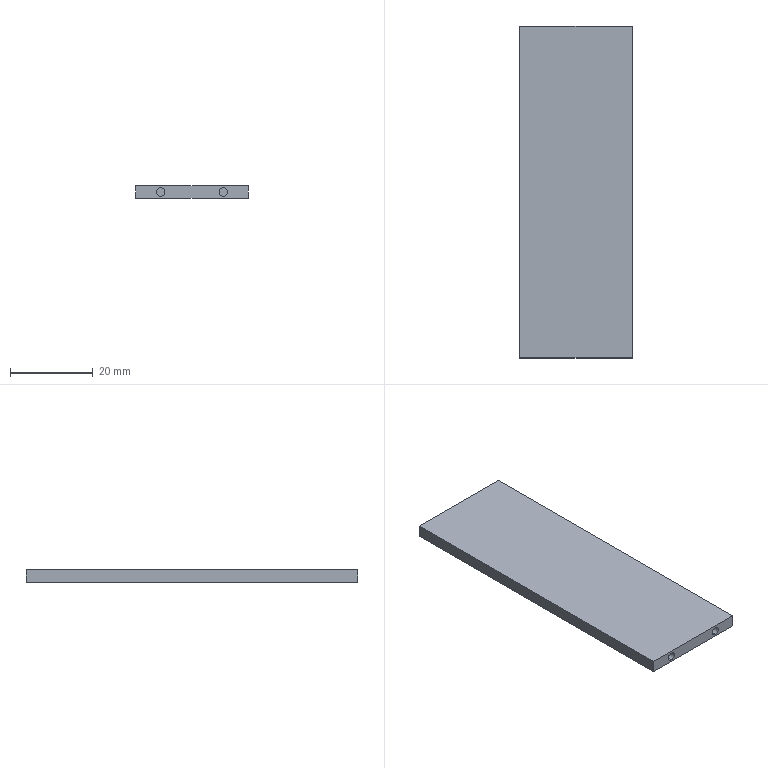Part | SolidWorks | features Cut 1, Extrusion 1 | 1 solid | 12 faces | box 27 x 80 x 3 mm | volume 6449 mm3 | plane 8 | cylinder 4 | commonest cylinder face diameters 2 x4
STEP:
#1=CARTESIAN_POINT('',(-28.957,-53.022,2.5));
#2=VERTEX_POINT('',#1);
#3=CARTESIAN_POINT('',(-28.957,-53.022,0.5));
#4=VERTEX_POINT('',#3);
#5=CARTESIAN_POINT('',(-28.957,-53.022,1.5));
#6=DIRECTION('',(0.,-1.,0.));
#7=DIRECTION('',(0.,0.,-1.));
#8=AXIS2_PLACEMENT_3D('',#5,#6,#7);
#9=CIRCLE('',#8,1.);
#10=EDGE_CURVE('',#2,#4,#9,.T.);
#11=ORIENTED_EDGE('',*,*,#10,.F.);
#12=CARTESIAN_POINT('',(-28.957,-58.022,2.5));
#13=VERTEX_POINT('',#12);
#14=CARTESIAN_POINT('',(-28.957,-53.022,2.5));
#15=DIRECTION('',(0.,-1.,0.));
#16=VECTOR('',#15,1000.);
#17=LINE('',#14,#16);
#18=EDGE_CURVE('',#2,#13,#17,.T.);
#19=ORIENTED_EDGE('',*,*,#18,.T.);
#20=CARTESIAN_POINT('',(-28.957,-58.022,0.5));
#21=VERTEX_POINT('',#20);
#22=CARTESIAN_POINT('',(-28.957,-58.022,1.5));
#23=DIRECTION('',(0.,1.,0.));
#24=DIRECTION('',(0.,0.,1.));
#25=AXIS2_PLACEMENT_3D('',#22,#23,#24);
#26=CIRCLE('',#25,1.);
#27=EDGE_CURVE('',#21,#13,#26,.T.);
#28=ORIENTED_EDGE('',*,*,#27,.F.);
#29=CARTESIAN_POINT('',(-28.957,-53.022,0.5));
#30=DIRECTION('',(0.,-1.,0.));
#31=VECTOR('',#30,1000.);
#32=LINE('',#29,#31);
#33=EDGE_CURVE('',#4,#21,#32,.T.);
#34=ORIENTED_EDGE('',*,*,#33,.F.);
#35=EDGE_LOOP('',(#11,#19,#28,#34));
#36=FACE_OUTER_BOUND('',#35,.T.);
#37=CARTESIAN_POINT('',(-28.957,-53.022,1.5));
#38=DIRECTION('',(0.,-1.,0.));
#39=DIRECTION('',(0.,0.,-1.));
#40=AXIS2_PLACEMENT_3D('',#37,#38,#39);
#41=CYLINDRICAL_SURFACE('',#40,1.);
#42=ADVANCED_FACE('',(#36),#41,.F.);
#43=CARTESIAN_POINT('',(-13.957,-53.022,2.5));
#44=VERTEX_POINT('',#43);
#45=CARTESIAN_POINT('',(-13.957,-53.022,0.5));
#46=VERTEX_POINT('',#45);
#47=CARTESIAN_POINT('',(-13.957,-53.022,1.5));
#48=DIRECTION('',(0.,-1.,0.));
#49=DIRECTION('',(0.,0.,-1.));
#50=AXIS2_PLACEMENT_3D('',#47,#48,#49);
#51=CIRCLE('',#50,1.);
#52=EDGE_CURVE('',#44,#46,#51,.T.);
#53=ORIENTED_EDGE('',*,*,#52,.F.);
#54=CARTESIAN_POINT('',(-13.957,-58.022,2.5));
#55=VERTEX_POINT('',#54);
#56=CARTESIAN_POINT('',(-13.957,-53.022,2.5));
#57=DIRECTION('',(0.,-1.,0.));
#58=VECTOR('',#57,1000.);
#59=LINE('',#56,#58);
#60=EDGE_CURVE('',#44,#55,#59,.T.);
#61=ORIENTED_EDGE('',*,*,#60,.T.);
#62=CARTESIAN_POINT('',(-13.957,-58.022,0.5));
#63=VERTEX_POINT('',#62);
#64=CARTESIAN_POINT('',(-13.957,-58.022,1.5));
#65=DIRECTION('',(0.,1.,0.));
#66=DIRECTION('',(0.,0.,1.));
#67=AXIS2_PLACEMENT_3D('',#64,#65,#66);
#68=CIRCLE('',#67,1.);
#69=EDGE_CURVE('',#63,#55,#68,.T.);
#70=ORIENTED_EDGE('',*,*,#69,.F.);
#71=CARTESIAN_POINT('',(-13.957,-53.022,0.5));
#72=DIRECTION('',(0.,-1.,0.));
#73=VECTOR('',#72,1000.);
#74=LINE('',#71,#73);
#75=EDGE_CURVE('',#46,#63,#74,.T.);
#76=ORIENTED_EDGE('',*,*,#75,.F.);
#77=EDGE_LOOP('',(#53,#61,#70,#76));
#78=FACE_OUTER_BOUND('',#77,.T.);
#79=CARTESIAN_POINT('',(-13.957,-53.022,1.5));
#80=DIRECTION('',(0.,-1.,0.));
#81=DIRECTION('',(0.,0.,-1.));
#82=AXIS2_PLACEMENT_3D('',#79,#80,#81);
#83=CYLINDRICAL_SURFACE('',#82,1.);
#84=ADVANCED_FACE('',(#78),#83,.F.);
#85=ORIENTED_EDGE('',*,*,#27,.T.);
#86=CARTESIAN_POINT('',(-28.957,-58.022,1.5));
#87=DIRECTION('',(0.,1.,0.));
#88=DIRECTION('',(0.,0.,1.));
#89=AXIS2_PLACEMENT_3D('',#86,#87,#88);
#90=CIRCLE('',#89,1.);
#91=EDGE_CURVE('',#13,#21,#90,.T.);
#92=ORIENTED_EDGE('',*,*,#91,.T.);
#93=EDGE_LOOP('',(#85,#92));
#94=FACE_BOUND('',#93,.T.);
#95=ORIENTED_EDGE('',*,*,#69,.T.);
#96=CARTESIAN_POINT('',(-13.957,-58.022,1.5));
#97=DIRECTION('',(0.,1.,0.));
#98=DIRECTION('',(0.,0.,1.));
#99=AXIS2_PLACEMENT_3D('',#96,#97,#98);
#100=CIRCLE('',#99,1.);
#101=EDGE_CURVE('',#55,#63,#100,.T.);
#102=ORIENTED_EDGE('',*,*,#101,.T.);
#103=EDGE_LOOP('',(#95,#102));
#104=FACE_BOUND('',#103,.T.);
#105=CARTESIAN_POINT('',(-34.957,-58.022,0.));
#106=VERTEX_POINT('',#105);
#107=CARTESIAN_POINT('',(-7.957,-58.022,0.));
#108=VERTEX_POINT('',#107);
#109=CARTESIAN_POINT('',(-34.957,-58.022,0.));
#110=DIRECTION('',(1.,0.,0.));
#111=VECTOR('',#110,1000.);
#112=LINE('',#109,#111);
#113=EDGE_CURVE('',#106,#108,#112,.T.);
#114=ORIENTED_EDGE('',*,*,#113,.T.);
#115=CARTESIAN_POINT('',(-7.957,-58.022,3.));
#116=VERTEX_POINT('',#115);
#117=CARTESIAN_POINT('',(-7.957,-58.022,3.));
#118=DIRECTION('',(0.,0.,-1.));
#119=VECTOR('',#118,1000.);
#120=LINE('',#117,#119);
#121=EDGE_CURVE('',#116,#108,#120,.T.);
#122=ORIENTED_EDGE('',*,*,#121,.F.);
#123=CARTESIAN_POINT('',(-34.957,-58.022,3.));
#124=VERTEX_POINT('',#123);
#125=CARTESIAN_POINT('',(-34.957,-58.022,3.));
#126=DIRECTION('',(1.,0.,0.));
#127=VECTOR('',#126,1000.);
#128=LINE('',#125,#127);
#129=EDGE_CURVE('',#124,#116,#128,.T.);
#130=ORIENTED_EDGE('',*,*,#129,.F.);
#131=CARTESIAN_POINT('',(-34.957,-58.022,3.));
#132=DIRECTION('',(0.,0.,-1.));
#133=VECTOR('',#132,1000.);
#134=LINE('',#131,#133);
#135=EDGE_CURVE('',#124,#106,#134,.T.);
#136=ORIENTED_EDGE('',*,*,#135,.T.);
#137=EDGE_LOOP('',(#114,#122,#130,#136));
#138=FACE_OUTER_BOUND('',#137,.T.);
#139=CARTESIAN_POINT('',(-34.957,-58.022,3.));
#140=DIRECTION('',(0.,1.,0.));
#141=DIRECTION('',(0.,0.,1.));
#142=AXIS2_PLACEMENT_3D('',#139,#140,#141);
#143=PLANE('',#142);
#144=ADVANCED_FACE('',(#94,#104,#138),#143,.F.);
#145=CARTESIAN_POINT('',(-7.957,21.978,0.));
#146=VERTEX_POINT('',#145);
#147=CARTESIAN_POINT('',(-7.957,-58.022,0.));
#148=DIRECTION('',(0.,1.,0.));
#149=VECTOR('',#148,1000.);
#150=LINE('',#147,#149);
#151=EDGE_CURVE('',#108,#146,#150,.T.);
#152=ORIENTED_EDGE('',*,*,#151,.T.);
#153=CARTESIAN_POINT('',(-7.957,21.978,3.));
#154=VERTEX_POINT('',#153);
#155=CARTESIAN_POINT('',(-7.957,21.978,3.));
#156=DIRECTION('',(0.,0.,-1.));
#157=VECTOR('',#156,1000.);
#158=LINE('',#155,#157);
#159=EDGE_CURVE('',#154,#146,#158,.T.);
#160=ORIENTED_EDGE('',*,*,#159,.F.);
#161=CARTESIAN_POINT('',(-7.957,-58.022,3.));
#162=DIRECTION('',(0.,1.,0.));
#163=VECTOR('',#162,1000.);
#164=LINE('',#161,#163);
#165=EDGE_CURVE('',#116,#154,#164,.T.);
#166=ORIENTED_EDGE('',*,*,#165,.F.);
#167=ORIENTED_EDGE('',*,*,#121,.T.);
#168=EDGE_LOOP('',(#152,#160,#166,#167));
#169=FACE_OUTER_BOUND('',#168,.T.);
#170=CARTESIAN_POINT('',(-7.957,-58.022,3.));
#171=DIRECTION('',(-1.,0.,0.));
#172=DIRECTION('',(0.,0.,1.));
#173=AXIS2_PLACEMENT_3D('',#170,#171,#172);
#174=PLANE('',#173);
#175=ADVANCED_FACE('',(#169),#174,.F.);
#176=CARTESIAN_POINT('',(-34.957,21.978,0.));
#177=VERTEX_POINT('',#176);
#178=CARTESIAN_POINT('',(-34.957,21.978,0.));
#179=DIRECTION('',(1.,0.,0.));
#180=VECTOR('',#179,1000.);
#181=LINE('',#178,#180);
#182=EDGE_CURVE('',#177,#146,#181,.T.);
#183=ORIENTED_EDGE('',*,*,#182,.F.);
#184=CARTESIAN_POINT('',(-34.957,21.978,3.));
#185=VERTEX_POINT('',#184);
#186=CARTESIAN_POINT('',(-34.957,21.978,3.));
#187=DIRECTION('',(0.,0.,-1.));
#188=VECTOR('',#187,1000.);
#189=LINE('',#186,#188);
#190=EDGE_CURVE('',#185,#177,#189,.T.);
#191=ORIENTED_EDGE('',*,*,#190,.F.);
#192=CARTESIAN_POINT('',(-34.957,21.978,3.));
#193=DIRECTION('',(1.,0.,0.));
#194=VECTOR('',#193,1000.);
#195=LINE('',#192,#194);
#196=EDGE_CURVE('',#185,#154,#195,.T.);
#197=ORIENTED_EDGE('',*,*,#196,.T.);
#198=ORIENTED_EDGE('',*,*,#159,.T.);
#199=EDGE_LOOP('',(#183,#191,#197,#198));
#200=FACE_OUTER_BOUND('',#199,.T.);
#201=CARTESIAN_POINT('',(-34.957,21.978,3.));
#202=DIRECTION('',(0.,1.,0.));
#203=DIRECTION('',(0.,0.,1.));
#204=AXIS2_PLACEMENT_3D('',#201,#202,#203);
#205=PLANE('',#204);
#206=ADVANCED_FACE('',(#200),#205,.T.);
#207=CARTESIAN_POINT('',(-34.957,-58.022,0.));
#208=DIRECTION('',(0.,1.,0.));
#209=VECTOR('',#208,1000.);
#210=LINE('',#207,#209);
#211=EDGE_CURVE('',#106,#177,#210,.T.);
#212=ORIENTED_EDGE('',*,*,#211,.F.);
#213=ORIENTED_EDGE('',*,*,#135,.F.);
#214=CARTESIAN_POINT('',(-34.957,-58.022,3.));
#215=DIRECTION('',(0.,1.,0.));
#216=VECTOR('',#215,1000.);
#217=LINE('',#214,#216);
#218=EDGE_CURVE('',#124,#185,#217,.T.);
#219=ORIENTED_EDGE('',*,*,#218,.T.);
#220=ORIENTED_EDGE('',*,*,#190,.T.);
#221=EDGE_LOOP('',(#212,#213,#219,#220));
#222=FACE_OUTER_BOUND('',#221,.T.);
#223=CARTESIAN_POINT('',(-34.957,-58.022,3.));
#224=DIRECTION('',(-1.,0.,0.));
#225=DIRECTION('',(0.,0.,1.));
#226=AXIS2_PLACEMENT_3D('',#223,#224,#225);
#227=PLANE('',#226);
#228=ADVANCED_FACE('',(#222),#227,.T.);
#229=ORIENTED_EDGE('',*,*,#129,.T.);
#230=ORIENTED_EDGE('',*,*,#165,.T.);
#231=ORIENTED_EDGE('',*,*,#196,.F.);
#232=ORIENTED_EDGE('',*,*,#218,.F.);
#233=EDGE_LOOP('',(#229,#230,#231,#232));
#234=FACE_OUTER_BOUND('',#233,.T.);
#235=CARTESIAN_POINT('',(0.,0.,3.));
#236=DIRECTION('',(0.,0.,1.));
#237=DIRECTION('',(1.,0.,0.));
#238=AXIS2_PLACEMENT_3D('',#235,#236,#237);
#239=PLANE('',#238);
#240=ADVANCED_FACE('',(#234),#239,.T.);
#241=ORIENTED_EDGE('',*,*,#113,.F.);
#242=ORIENTED_EDGE('',*,*,#211,.T.);
#243=ORIENTED_EDGE('',*,*,#182,.T.);
#244=ORIENTED_EDGE('',*,*,#151,.F.);
#245=EDGE_LOOP('',(#241,#242,#243,#244));
#246=FACE_OUTER_BOUND('',#245,.T.);
#247=CARTESIAN_POINT('',(0.,0.,0.));
#248=DIRECTION('',(0.,0.,1.));
#249=DIRECTION('',(1.,0.,0.));
#250=AXIS2_PLACEMENT_3D('',#247,#248,#249);
#251=PLANE('',#250);
#252=ADVANCED_FACE('',(#246),#251,.F.);
#253=ORIENTED_EDGE('',*,*,#60,.F.);
#254=CARTESIAN_POINT('',(-13.957,-53.022,1.5));
#255=DIRECTION('',(0.,-1.,0.));
#256=DIRECTION('',(0.,0.,-1.));
#257=AXIS2_PLACEMENT_3D('',#254,#255,#256);
#258=CIRCLE('',#257,1.);
#259=EDGE_CURVE('',#46,#44,#258,.T.);
#260=ORIENTED_EDGE('',*,*,#259,.F.);
#261=ORIENTED_EDGE('',*,*,#75,.T.);
#262=ORIENTED_EDGE('',*,*,#101,.F.);
#263=EDGE_LOOP('',(#253,#260,#261,#262));
#264=FACE_OUTER_BOUND('',#263,.T.);
#265=CARTESIAN_POINT('',(-13.957,-53.022,1.5));
#266=DIRECTION('',(0.,-1.,0.));
#267=DIRECTION('',(0.,0.,-1.));
#268=AXIS2_PLACEMENT_3D('',#265,#266,#267);
#269=CYLINDRICAL_SURFACE('',#268,1.);
#270=ADVANCED_FACE('',(#264),#269,.F.);
#271=ORIENTED_EDGE('',*,*,#259,.T.);
#272=ORIENTED_EDGE('',*,*,#52,.T.);
#273=EDGE_LOOP('',(#271,#272));
#274=FACE_OUTER_BOUND('',#273,.T.);
#275=CARTESIAN_POINT('',(-13.957,-53.022,1.5));
#276=DIRECTION('',(0.,-1.,0.));
#277=DIRECTION('',(0.,0.,-1.));
#278=AXIS2_PLACEMENT_3D('',#275,#276,#277);
#279=PLANE('',#278);
#280=ADVANCED_FACE('',(#274),#279,.T.);
#281=ORIENTED_EDGE('',*,*,#18,.F.);
#282=CARTESIAN_POINT('',(-28.957,-53.022,1.5));
#283=DIRECTION('',(0.,-1.,0.));
#284=DIRECTION('',(0.,0.,-1.));
#285=AXIS2_PLACEMENT_3D('',#282,#283,#284);
#286=CIRCLE('',#285,1.);
#287=EDGE_CURVE('',#4,#2,#286,.T.);
#288=ORIENTED_EDGE('',*,*,#287,.F.);
#289=ORIENTED_EDGE('',*,*,#33,.T.);
#290=ORIENTED_EDGE('',*,*,#91,.F.);
#291=EDGE_LOOP('',(#281,#288,#289,#290));
#292=FACE_OUTER_BOUND('',#291,.T.);
#293=CARTESIAN_POINT('',(-28.957,-53.022,1.5));
#294=DIRECTION('',(0.,-1.,0.));
#295=DIRECTION('',(0.,0.,-1.));
#296=AXIS2_PLACEMENT_3D('',#293,#294,#295);
#297=CYLINDRICAL_SURFACE('',#296,1.);
#298=ADVANCED_FACE('',(#292),#297,.F.);
#299=ORIENTED_EDGE('',*,*,#287,.T.);
#300=ORIENTED_EDGE('',*,*,#10,.T.);
#301=EDGE_LOOP('',(#299,#300));
#302=FACE_OUTER_BOUND('',#301,.T.);
#303=CARTESIAN_POINT('',(-28.957,-53.022,1.5));
#304=DIRECTION('',(0.,-1.,0.));
#305=DIRECTION('',(0.,0.,-1.));
#306=AXIS2_PLACEMENT_3D('',#303,#304,#305);
#307=PLANE('',#306);
#308=ADVANCED_FACE('',(#302),#307,.T.);
#309=CLOSED_SHELL('',(#42,#84,#144,#175,#206,#228,#240,#252,#270,#280,#298,#308));
#310=MANIFOLD_SOLID_BREP('',#309);
#311=CARTESIAN_POINT('',(0.,0.,0.));
#312=DIRECTION('',(0.,0.,1.));
#313=DIRECTION('',(1.,0.,0.));
#314=AXIS2_PLACEMENT_3D('',#311,#312,#313);
#315=(LENGTH_UNIT()NAMED_UNIT(*)SI_UNIT(.MILLI.,.METRE.));
#316=UNCERTAINTY_MEASURE_WITH_UNIT(LENGTH_MEASURE(0.00001),#315,'','');
#317=(NAMED_UNIT(*)PLANE_ANGLE_UNIT()SI_UNIT($,.RADIAN.));
#318=(NAMED_UNIT(*)SI_UNIT($,.STERADIAN.)SOLID_ANGLE_UNIT());
#319=(GEOMETRIC_REPRESENTATION_CONTEXT(3)GLOBAL_UNCERTAINTY_ASSIGNED_CONTEXT((#316))GLOBAL_UNIT_ASSIGNED_CONTEXT((#315,#317,#318))REPRESENTATION_CONTEXT('',''));
#320=ADVANCED_BREP_SHAPE_REPRESENTATION('',(#310,#314),#319);